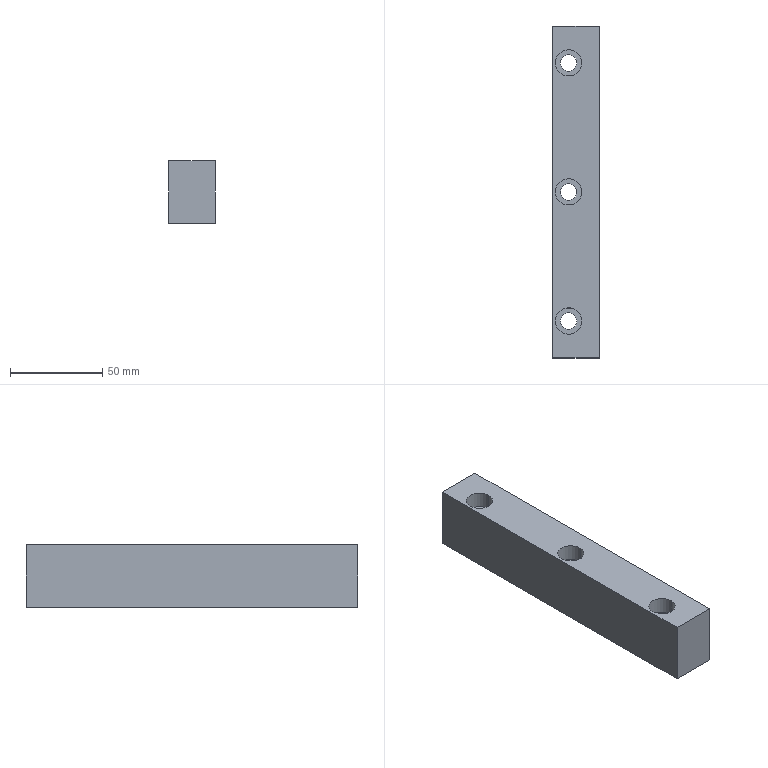Part | Creo | 1 solid | 21 faces | box 25 x 180 x 34 mm | volume 143923 mm3 | cylinder 12 | plane 9 | commonest cylinder face diameters 9 x6 14.25 x6
STEP:
#1=CARTESIAN_POINT('',(0.,0.,0.));
#2=DIRECTION('',(0.,0.,1.));
#3=DIRECTION('',(1.,0.,0.));
#4=AXIS2_PLACEMENT_3D('',#1,#2,#3);
#5=CARTESIAN_POINT('',(148.764,125.373,-29.441));
#6=VERTEX_POINT('',#5);
#7=CARTESIAN_POINT('',(173.764,125.373,-29.441));
#8=VERTEX_POINT('',#7);
#9=CARTESIAN_POINT('',(148.764,125.373,-29.441));
#10=DIRECTION('',(1.,0.,0.));
#11=VECTOR('',#10,25.);
#12=LINE('',#9,#11);
#13=EDGE_CURVE('',#6,#8,#12,.T.);
#14=ORIENTED_EDGE('',*,*,#13,.F.);
#15=CARTESIAN_POINT('',(148.764,305.373,-29.441));
#16=VERTEX_POINT('',#15);
#17=CARTESIAN_POINT('',(148.764,125.373,-29.441));
#18=DIRECTION('',(0.,1.,0.));
#19=VECTOR('',#18,180.);
#20=LINE('',#17,#19);
#21=EDGE_CURVE('',#6,#16,#20,.T.);
#22=ORIENTED_EDGE('',*,*,#21,.T.);
#23=CARTESIAN_POINT('',(173.764,305.373,-29.441));
#24=VERTEX_POINT('',#23);
#25=CARTESIAN_POINT('',(148.764,305.373,-29.441));
#26=DIRECTION('',(1.,0.,0.));
#27=VECTOR('',#26,25.);
#28=LINE('',#25,#27);
#29=EDGE_CURVE('',#16,#24,#28,.T.);
#30=ORIENTED_EDGE('',*,*,#29,.T.);
#31=CARTESIAN_POINT('',(173.764,125.373,-29.441));
#32=DIRECTION('',(0.,1.,0.));
#33=VECTOR('',#32,180.);
#34=LINE('',#31,#33);
#35=EDGE_CURVE('',#8,#24,#34,.T.);
#36=ORIENTED_EDGE('',*,*,#35,.F.);
#37=EDGE_LOOP('',(#14,#22,#30,#36));
#38=FACE_OUTER_BOUND('',#37,.F.);
#39=CARTESIAN_POINT('',(150.139,285.373,-29.441));
#40=VERTEX_POINT('',#39);
#41=CARTESIAN_POINT('',(164.389,285.373,-29.441));
#42=VERTEX_POINT('',#41);
#43=CARTESIAN_POINT('',(157.264,285.373,-29.441));
#44=DIRECTION('',(0.,0.,-1.));
#45=DIRECTION('',(-1.,0.,0.));
#46=AXIS2_PLACEMENT_3D('',#43,#44,#45);
#47=CIRCLE('',#46,7.125);
#48=EDGE_CURVE('',#40,#42,#47,.T.);
#49=ORIENTED_EDGE('',*,*,#48,.F.);
#50=CARTESIAN_POINT('',(157.264,285.373,-29.441));
#51=DIRECTION('',(0.,0.,-1.));
#52=DIRECTION('',(1.,0.,0.));
#53=AXIS2_PLACEMENT_3D('',#50,#51,#52);
#54=CIRCLE('',#53,7.125);
#55=EDGE_CURVE('',#42,#40,#54,.T.);
#56=ORIENTED_EDGE('',*,*,#55,.F.);
#57=EDGE_LOOP('',(#49,#56));
#58=FACE_BOUND('',#57,.F.);
#59=CARTESIAN_POINT('',(150.139,145.373,-29.441));
#60=VERTEX_POINT('',#59);
#61=CARTESIAN_POINT('',(164.389,145.373,-29.441));
#62=VERTEX_POINT('',#61);
#63=CARTESIAN_POINT('',(157.264,145.373,-29.441));
#64=DIRECTION('',(0.,0.,-1.));
#65=DIRECTION('',(-1.,0.,0.));
#66=AXIS2_PLACEMENT_3D('',#63,#64,#65);
#67=CIRCLE('',#66,7.125);
#68=EDGE_CURVE('',#60,#62,#67,.T.);
#69=ORIENTED_EDGE('',*,*,#68,.F.);
#70=CARTESIAN_POINT('',(157.264,145.373,-29.441));
#71=DIRECTION('',(0.,0.,-1.));
#72=DIRECTION('',(1.,0.,0.));
#73=AXIS2_PLACEMENT_3D('',#70,#71,#72);
#74=CIRCLE('',#73,7.125);
#75=EDGE_CURVE('',#62,#60,#74,.T.);
#76=ORIENTED_EDGE('',*,*,#75,.F.);
#77=EDGE_LOOP('',(#69,#76));
#78=FACE_BOUND('',#77,.F.);
#79=CARTESIAN_POINT('',(150.139,215.373,-29.441));
#80=VERTEX_POINT('',#79);
#81=CARTESIAN_POINT('',(164.389,215.373,-29.441));
#82=VERTEX_POINT('',#81);
#83=CARTESIAN_POINT('',(157.264,215.373,-29.441));
#84=DIRECTION('',(0.,0.,-1.));
#85=DIRECTION('',(-1.,0.,0.));
#86=AXIS2_PLACEMENT_3D('',#83,#84,#85);
#87=CIRCLE('',#86,7.125);
#88=EDGE_CURVE('',#80,#82,#87,.T.);
#89=ORIENTED_EDGE('',*,*,#88,.F.);
#90=CARTESIAN_POINT('',(157.264,215.373,-29.441));
#91=DIRECTION('',(0.,0.,-1.));
#92=DIRECTION('',(1.,0.,0.));
#93=AXIS2_PLACEMENT_3D('',#90,#91,#92);
#94=CIRCLE('',#93,7.125);
#95=EDGE_CURVE('',#82,#80,#94,.T.);
#96=ORIENTED_EDGE('',*,*,#95,.F.);
#97=EDGE_LOOP('',(#89,#96));
#98=FACE_BOUND('',#97,.F.);
#99=CARTESIAN_POINT('',(439.623,319.968,-29.441));
#100=DIRECTION('',(0.,0.,-1.));
#101=DIRECTION('',(-1.,0.,0.));
#102=AXIS2_PLACEMENT_3D('',#99,#100,#101);
#103=PLANE('',#102);
#104=ADVANCED_FACE('',(#38,#58,#78,#98),#103,.F.);
#105=ORIENTED_EDGE('',*,*,#48,.T.);
#106=CARTESIAN_POINT('',(164.389,285.373,-38.441));
#107=VERTEX_POINT('',#106);
#108=CARTESIAN_POINT('',(164.389,285.373,-38.441));
#109=DIRECTION('',(0.,0.,1.));
#110=VECTOR('',#109,9.);
#111=LINE('',#108,#110);
#112=EDGE_CURVE('',#107,#42,#111,.T.);
#113=ORIENTED_EDGE('',*,*,#112,.F.);
#114=CARTESIAN_POINT('',(150.139,285.373,-38.441));
#115=VERTEX_POINT('',#114);
#116=CARTESIAN_POINT('',(157.264,285.373,-38.441));
#117=DIRECTION('',(0.,0.,1.));
#118=DIRECTION('',(1.,0.,0.));
#119=AXIS2_PLACEMENT_3D('',#116,#117,#118);
#120=CIRCLE('',#119,7.125);
#121=EDGE_CURVE('',#107,#115,#120,.T.);
#122=ORIENTED_EDGE('',*,*,#121,.T.);
#123=CARTESIAN_POINT('',(150.139,285.373,-38.441));
#124=DIRECTION('',(0.,0.,1.));
#125=VECTOR('',#124,9.);
#126=LINE('',#123,#125);
#127=EDGE_CURVE('',#115,#40,#126,.T.);
#128=ORIENTED_EDGE('',*,*,#127,.T.);
#129=EDGE_LOOP('',(#105,#113,#122,#128));
#130=FACE_OUTER_BOUND('',#129,.F.);
#131=CARTESIAN_POINT('',(157.264,285.373,-38.441));
#132=DIRECTION('',(0.,0.,1.));
#133=DIRECTION('',(1.,0.,0.));
#134=AXIS2_PLACEMENT_3D('',#131,#132,#133);
#135=CYLINDRICAL_SURFACE('',#134,7.125);
#136=ADVANCED_FACE('',(#130),#135,.F.);
#137=ORIENTED_EDGE('',*,*,#55,.T.);
#138=ORIENTED_EDGE('',*,*,#127,.F.);
#139=CARTESIAN_POINT('',(157.264,285.373,-38.441));
#140=DIRECTION('',(0.,0.,1.));
#141=DIRECTION('',(-1.,0.,0.));
#142=AXIS2_PLACEMENT_3D('',#139,#140,#141);
#143=CIRCLE('',#142,7.125);
#144=EDGE_CURVE('',#115,#107,#143,.T.);
#145=ORIENTED_EDGE('',*,*,#144,.T.);
#146=ORIENTED_EDGE('',*,*,#112,.T.);
#147=EDGE_LOOP('',(#137,#138,#145,#146));
#148=FACE_OUTER_BOUND('',#147,.F.);
#149=CARTESIAN_POINT('',(157.264,285.373,-38.441));
#150=DIRECTION('',(0.,0.,1.));
#151=DIRECTION('',(1.,0.,0.));
#152=AXIS2_PLACEMENT_3D('',#149,#150,#151);
#153=CYLINDRICAL_SURFACE('',#152,7.125);
#154=ADVANCED_FACE('',(#148),#153,.F.);
#155=ORIENTED_EDGE('',*,*,#144,.F.);
#156=ORIENTED_EDGE('',*,*,#121,.F.);
#157=EDGE_LOOP('',(#155,#156));
#158=FACE_OUTER_BOUND('',#157,.F.);
#159=CARTESIAN_POINT('',(161.764,285.373,-38.441));
#160=VERTEX_POINT('',#159);
#161=CARTESIAN_POINT('',(152.764,285.373,-38.441));
#162=VERTEX_POINT('',#161);
#163=CARTESIAN_POINT('',(157.264,285.373,-38.441));
#164=DIRECTION('',(0.,0.,-1.));
#165=DIRECTION('',(1.,0.,0.));
#166=AXIS2_PLACEMENT_3D('',#163,#164,#165);
#167=CIRCLE('',#166,4.5);
#168=EDGE_CURVE('',#160,#162,#167,.T.);
#169=ORIENTED_EDGE('',*,*,#168,.F.);
#170=CARTESIAN_POINT('',(157.264,285.373,-38.441));
#171=DIRECTION('',(0.,0.,-1.));
#172=DIRECTION('',(-1.,0.,0.));
#173=AXIS2_PLACEMENT_3D('',#170,#171,#172);
#174=CIRCLE('',#173,4.5);
#175=EDGE_CURVE('',#162,#160,#174,.T.);
#176=ORIENTED_EDGE('',*,*,#175,.F.);
#177=EDGE_LOOP('',(#169,#176));
#178=FACE_BOUND('',#177,.F.);
#179=CARTESIAN_POINT('',(157.264,285.373,-38.441));
#180=DIRECTION('',(0.,0.,-1.));
#181=DIRECTION('',(-1.,0.,0.));
#182=AXIS2_PLACEMENT_3D('',#179,#180,#181);
#183=PLANE('',#182);
#184=ADVANCED_FACE('',(#158,#178),#183,.F.);
#185=CARTESIAN_POINT('',(152.764,285.373,-63.441));
#186=VERTEX_POINT('',#185);
#187=CARTESIAN_POINT('',(161.764,285.373,-63.441));
#188=VERTEX_POINT('',#187);
#189=CARTESIAN_POINT('',(157.264,285.373,-63.441));
#190=DIRECTION('',(0.,0.,1.));
#191=DIRECTION('',(-1.,0.,0.));
#192=AXIS2_PLACEMENT_3D('',#189,#190,#191);
#193=CIRCLE('',#192,4.5);
#194=EDGE_CURVE('',#186,#188,#193,.T.);
#195=ORIENTED_EDGE('',*,*,#194,.T.);
#196=CARTESIAN_POINT('',(161.764,285.373,-38.441));
#197=DIRECTION('',(0.,0.,-1.));
#198=VECTOR('',#197,25.);
#199=LINE('',#196,#198);
#200=EDGE_CURVE('',#160,#188,#199,.T.);
#201=ORIENTED_EDGE('',*,*,#200,.F.);
#202=ORIENTED_EDGE('',*,*,#168,.T.);
#203=CARTESIAN_POINT('',(152.764,285.373,-38.441));
#204=DIRECTION('',(0.,0.,-1.));
#205=VECTOR('',#204,25.);
#206=LINE('',#203,#205);
#207=EDGE_CURVE('',#162,#186,#206,.T.);
#208=ORIENTED_EDGE('',*,*,#207,.T.);
#209=EDGE_LOOP('',(#195,#201,#202,#208));
#210=FACE_OUTER_BOUND('',#209,.F.);
#211=CARTESIAN_POINT('',(157.264,285.373,-38.441));
#212=DIRECTION('',(0.,0.,-1.));
#213=DIRECTION('',(-1.,0.,0.));
#214=AXIS2_PLACEMENT_3D('',#211,#212,#213);
#215=CYLINDRICAL_SURFACE('',#214,4.5);
#216=ADVANCED_FACE('',(#210),#215,.F.);
#217=CARTESIAN_POINT('',(148.764,125.373,-63.441));
#218=VERTEX_POINT('',#217);
#219=CARTESIAN_POINT('',(173.764,125.373,-63.441));
#220=VERTEX_POINT('',#219);
#221=CARTESIAN_POINT('',(148.764,125.373,-63.441));
#222=DIRECTION('',(1.,0.,0.));
#223=VECTOR('',#222,25.);
#224=LINE('',#221,#223);
#225=EDGE_CURVE('',#218,#220,#224,.T.);
#226=ORIENTED_EDGE('',*,*,#225,.T.);
#227=CARTESIAN_POINT('',(173.764,305.373,-63.441));
#228=VERTEX_POINT('',#227);
#229=CARTESIAN_POINT('',(173.764,125.373,-63.441));
#230=DIRECTION('',(0.,1.,0.));
#231=VECTOR('',#230,180.);
#232=LINE('',#229,#231);
#233=EDGE_CURVE('',#220,#228,#232,.T.);
#234=ORIENTED_EDGE('',*,*,#233,.T.);
#235=CARTESIAN_POINT('',(148.764,305.373,-63.441));
#236=VERTEX_POINT('',#235);
#237=CARTESIAN_POINT('',(148.764,305.373,-63.441));
#238=DIRECTION('',(1.,0.,0.));
#239=VECTOR('',#238,25.);
#240=LINE('',#237,#239);
#241=EDGE_CURVE('',#236,#228,#240,.T.);
#242=ORIENTED_EDGE('',*,*,#241,.F.);
#243=CARTESIAN_POINT('',(148.764,125.373,-63.441));
#244=DIRECTION('',(0.,1.,0.));
#245=VECTOR('',#244,180.);
#246=LINE('',#243,#245);
#247=EDGE_CURVE('',#218,#236,#246,.T.);
#248=ORIENTED_EDGE('',*,*,#247,.F.);
#249=EDGE_LOOP('',(#226,#234,#242,#248));
#250=FACE_OUTER_BOUND('',#249,.F.);
#251=CARTESIAN_POINT('',(157.264,285.373,-63.441));
#252=DIRECTION('',(0.,0.,1.));
#253=DIRECTION('',(1.,0.,0.));
#254=AXIS2_PLACEMENT_3D('',#251,#252,#253);
#255=CIRCLE('',#254,4.5);
#256=EDGE_CURVE('',#188,#186,#255,.T.);
#257=ORIENTED_EDGE('',*,*,#256,.F.);
#258=ORIENTED_EDGE('',*,*,#194,.F.);
#259=EDGE_LOOP('',(#257,#258));
#260=FACE_BOUND('',#259,.F.);
#261=CARTESIAN_POINT('',(161.764,145.373,-63.441));
#262=VERTEX_POINT('',#261);
#263=CARTESIAN_POINT('',(152.764,145.373,-63.441));
#264=VERTEX_POINT('',#263);
#265=CARTESIAN_POINT('',(157.264,145.373,-63.441));
#266=DIRECTION('',(0.,0.,1.));
#267=DIRECTION('',(1.,0.,0.));
#268=AXIS2_PLACEMENT_3D('',#265,#266,#267);
#269=CIRCLE('',#268,4.5);
#270=EDGE_CURVE('',#262,#264,#269,.T.);
#271=ORIENTED_EDGE('',*,*,#270,.F.);
#272=CARTESIAN_POINT('',(157.264,145.373,-63.441));
#273=DIRECTION('',(0.,0.,1.));
#274=DIRECTION('',(-1.,0.,0.));
#275=AXIS2_PLACEMENT_3D('',#272,#273,#274);
#276=CIRCLE('',#275,4.5);
#277=EDGE_CURVE('',#264,#262,#276,.T.);
#278=ORIENTED_EDGE('',*,*,#277,.F.);
#279=EDGE_LOOP('',(#271,#278));
#280=FACE_BOUND('',#279,.F.);
#281=CARTESIAN_POINT('',(161.764,215.373,-63.441));
#282=VERTEX_POINT('',#281);
#283=CARTESIAN_POINT('',(152.764,215.373,-63.441));
#284=VERTEX_POINT('',#283);
#285=CARTESIAN_POINT('',(157.264,215.373,-63.441));
#286=DIRECTION('',(0.,0.,1.));
#287=DIRECTION('',(1.,0.,0.));
#288=AXIS2_PLACEMENT_3D('',#285,#286,#287);
#289=CIRCLE('',#288,4.5);
#290=EDGE_CURVE('',#282,#284,#289,.T.);
#291=ORIENTED_EDGE('',*,*,#290,.F.);
#292=CARTESIAN_POINT('',(157.264,215.373,-63.441));
#293=DIRECTION('',(0.,0.,1.));
#294=DIRECTION('',(-1.,0.,0.));
#295=AXIS2_PLACEMENT_3D('',#292,#293,#294);
#296=CIRCLE('',#295,4.5);
#297=EDGE_CURVE('',#284,#282,#296,.T.);
#298=ORIENTED_EDGE('',*,*,#297,.F.);
#299=EDGE_LOOP('',(#291,#298));
#300=FACE_BOUND('',#299,.F.);
#301=CARTESIAN_POINT('',(439.623,319.968,-63.441));
#302=DIRECTION('',(0.,0.,-1.));
#303=DIRECTION('',(-1.,0.,0.));
#304=AXIS2_PLACEMENT_3D('',#301,#302,#303);
#305=PLANE('',#304);
#306=ADVANCED_FACE('',(#250,#260,#280,#300),#305,.T.);
#307=ORIENTED_EDGE('',*,*,#290,.T.);
#308=CARTESIAN_POINT('',(152.764,215.373,-38.441));
#309=VERTEX_POINT('',#308);
#310=CARTESIAN_POINT('',(152.764,215.373,-38.441));
#311=DIRECTION('',(0.,0.,-1.));
#312=VECTOR('',#311,25.);
#313=LINE('',#310,#312);
#314=EDGE_CURVE('',#309,#284,#313,.T.);
#315=ORIENTED_EDGE('',*,*,#314,.F.);
#316=CARTESIAN_POINT('',(161.764,215.373,-38.441));
#317=VERTEX_POINT('',#316);
#318=CARTESIAN_POINT('',(157.264,215.373,-38.441));
#319=DIRECTION('',(0.,0.,-1.));
#320=DIRECTION('',(-1.,0.,0.));
#321=AXIS2_PLACEMENT_3D('',#318,#319,#320);
#322=CIRCLE('',#321,4.5);
#323=EDGE_CURVE('',#309,#317,#322,.T.);
#324=ORIENTED_EDGE('',*,*,#323,.T.);
#325=CARTESIAN_POINT('',(161.764,215.373,-38.441));
#326=DIRECTION('',(0.,0.,-1.));
#327=VECTOR('',#326,25.);
#328=LINE('',#325,#327);
#329=EDGE_CURVE('',#317,#282,#328,.T.);
#330=ORIENTED_EDGE('',*,*,#329,.T.);
#331=EDGE_LOOP('',(#307,#315,#324,#330));
#332=FACE_OUTER_BOUND('',#331,.F.);
#333=CARTESIAN_POINT('',(157.264,215.373,-38.441));
#334=DIRECTION('',(0.,0.,-1.));
#335=DIRECTION('',(-1.,0.,0.));
#336=AXIS2_PLACEMENT_3D('',#333,#334,#335);
#337=CYLINDRICAL_SURFACE('',#336,4.5);
#338=ADVANCED_FACE('',(#332),#337,.F.);
#339=ORIENTED_EDGE('',*,*,#297,.T.);
#340=ORIENTED_EDGE('',*,*,#329,.F.);
#341=CARTESIAN_POINT('',(157.264,215.373,-38.441));
#342=DIRECTION('',(0.,0.,-1.));
#343=DIRECTION('',(1.,0.,0.));
#344=AXIS2_PLACEMENT_3D('',#341,#342,#343);
#345=CIRCLE('',#344,4.5);
#346=EDGE_CURVE('',#317,#309,#345,.T.);
#347=ORIENTED_EDGE('',*,*,#346,.T.);
#348=ORIENTED_EDGE('',*,*,#314,.T.);
#349=EDGE_LOOP('',(#339,#340,#347,#348));
#350=FACE_OUTER_BOUND('',#349,.F.);
#351=CARTESIAN_POINT('',(157.264,215.373,-38.441));
#352=DIRECTION('',(0.,0.,-1.));
#353=DIRECTION('',(-1.,0.,0.));
#354=AXIS2_PLACEMENT_3D('',#351,#352,#353);
#355=CYLINDRICAL_SURFACE('',#354,4.5);
#356=ADVANCED_FACE('',(#350),#355,.F.);
#357=CARTESIAN_POINT('',(150.139,215.373,-38.441));
#358=VERTEX_POINT('',#357);
#359=CARTESIAN_POINT('',(164.389,215.373,-38.441));
#360=VERTEX_POINT('',#359);
#361=CARTESIAN_POINT('',(157.264,215.373,-38.441));
#362=DIRECTION('',(0.,0.,1.));
#363=DIRECTION('',(-1.,0.,0.));
#364=AXIS2_PLACEMENT_3D('',#361,#362,#363);
#365=CIRCLE('',#364,7.125);
#366=EDGE_CURVE('',#358,#360,#365,.T.);
#367=ORIENTED_EDGE('',*,*,#366,.F.);
#368=CARTESIAN_POINT('',(157.264,215.373,-38.441));
#369=DIRECTION('',(0.,0.,1.));
#370=DIRECTION('',(1.,0.,0.));
#371=AXIS2_PLACEMENT_3D('',#368,#369,#370);
#372=CIRCLE('',#371,7.125);
#373=EDGE_CURVE('',#360,#358,#372,.T.);
#374=ORIENTED_EDGE('',*,*,#373,.F.);
#375=EDGE_LOOP('',(#367,#374));
#376=FACE_OUTER_BOUND('',#375,.F.);
#377=ORIENTED_EDGE('',*,*,#346,.F.);
#378=ORIENTED_EDGE('',*,*,#323,.F.);
#379=EDGE_LOOP('',(#377,#378));
#380=FACE_BOUND('',#379,.F.);
#381=CARTESIAN_POINT('',(157.264,215.373,-38.441));
#382=DIRECTION('',(0.,0.,-1.));
#383=DIRECTION('',(-1.,0.,0.));
#384=AXIS2_PLACEMENT_3D('',#381,#382,#383);
#385=PLANE('',#384);
#386=ADVANCED_FACE('',(#376,#380),#385,.F.);
#387=ORIENTED_EDGE('',*,*,#95,.T.);
#388=CARTESIAN_POINT('',(150.139,215.373,-38.441));
#389=DIRECTION('',(0.,0.,1.));
#390=VECTOR('',#389,9.);
#391=LINE('',#388,#390);
#392=EDGE_CURVE('',#358,#80,#391,.T.);
#393=ORIENTED_EDGE('',*,*,#392,.F.);
#394=ORIENTED_EDGE('',*,*,#366,.T.);
#395=CARTESIAN_POINT('',(164.389,215.373,-38.441));
#396=DIRECTION('',(0.,0.,1.));
#397=VECTOR('',#396,9.);
#398=LINE('',#395,#397);
#399=EDGE_CURVE('',#360,#82,#398,.T.);
#400=ORIENTED_EDGE('',*,*,#399,.T.);
#401=EDGE_LOOP('',(#387,#393,#394,#400));
#402=FACE_OUTER_BOUND('',#401,.F.);
#403=CARTESIAN_POINT('',(157.264,215.373,-38.441));
#404=DIRECTION('',(0.,0.,1.));
#405=DIRECTION('',(1.,0.,0.));
#406=AXIS2_PLACEMENT_3D('',#403,#404,#405);
#407=CYLINDRICAL_SURFACE('',#406,7.125);
#408=ADVANCED_FACE('',(#402),#407,.F.);
#409=ORIENTED_EDGE('',*,*,#88,.T.);
#410=ORIENTED_EDGE('',*,*,#399,.F.);
#411=ORIENTED_EDGE('',*,*,#373,.T.);
#412=ORIENTED_EDGE('',*,*,#392,.T.);
#413=EDGE_LOOP('',(#409,#410,#411,#412));
#414=FACE_OUTER_BOUND('',#413,.F.);
#415=CARTESIAN_POINT('',(157.264,215.373,-38.441));
#416=DIRECTION('',(0.,0.,1.));
#417=DIRECTION('',(1.,0.,0.));
#418=AXIS2_PLACEMENT_3D('',#415,#416,#417);
#419=CYLINDRICAL_SURFACE('',#418,7.125);
#420=ADVANCED_FACE('',(#414),#419,.F.);
#421=ORIENTED_EDGE('',*,*,#256,.T.);
#422=ORIENTED_EDGE('',*,*,#207,.F.);
#423=ORIENTED_EDGE('',*,*,#175,.T.);
#424=ORIENTED_EDGE('',*,*,#200,.T.);
#425=EDGE_LOOP('',(#421,#422,#423,#424));
#426=FACE_OUTER_BOUND('',#425,.F.);
#427=CARTESIAN_POINT('',(157.264,285.373,-38.441));
#428=DIRECTION('',(0.,0.,-1.));
#429=DIRECTION('',(-1.,0.,0.));
#430=AXIS2_PLACEMENT_3D('',#427,#428,#429);
#431=CYLINDRICAL_SURFACE('',#430,4.5);
#432=ADVANCED_FACE('',(#426),#431,.F.);
#433=ORIENTED_EDGE('',*,*,#270,.T.);
#434=CARTESIAN_POINT('',(152.764,145.373,-38.441));
#435=VERTEX_POINT('',#434);
#436=CARTESIAN_POINT('',(152.764,145.373,-38.441));
#437=DIRECTION('',(0.,0.,-1.));
#438=VECTOR('',#437,25.);
#439=LINE('',#436,#438);
#440=EDGE_CURVE('',#435,#264,#439,.T.);
#441=ORIENTED_EDGE('',*,*,#440,.F.);
#442=CARTESIAN_POINT('',(161.764,145.373,-38.441));
#443=VERTEX_POINT('',#442);
#444=CARTESIAN_POINT('',(157.264,145.373,-38.441));
#445=DIRECTION('',(0.,0.,-1.));
#446=DIRECTION('',(-1.,0.,0.));
#447=AXIS2_PLACEMENT_3D('',#444,#445,#446);
#448=CIRCLE('',#447,4.5);
#449=EDGE_CURVE('',#435,#443,#448,.T.);
#450=ORIENTED_EDGE('',*,*,#449,.T.);
#451=CARTESIAN_POINT('',(161.764,145.373,-38.441));
#452=DIRECTION('',(0.,0.,-1.));
#453=VECTOR('',#452,25.);
#454=LINE('',#451,#453);
#455=EDGE_CURVE('',#443,#262,#454,.T.);
#456=ORIENTED_EDGE('',*,*,#455,.T.);
#457=EDGE_LOOP('',(#433,#441,#450,#456));
#458=FACE_OUTER_BOUND('',#457,.F.);
#459=CARTESIAN_POINT('',(157.264,145.373,-38.441));
#460=DIRECTION('',(0.,0.,-1.));
#461=DIRECTION('',(-1.,0.,0.));
#462=AXIS2_PLACEMENT_3D('',#459,#460,#461);
#463=CYLINDRICAL_SURFACE('',#462,4.5);
#464=ADVANCED_FACE('',(#458),#463,.F.);
#465=ORIENTED_EDGE('',*,*,#277,.T.);
#466=ORIENTED_EDGE('',*,*,#455,.F.);
#467=CARTESIAN_POINT('',(157.264,145.373,-38.441));
#468=DIRECTION('',(0.,0.,-1.));
#469=DIRECTION('',(1.,0.,0.));
#470=AXIS2_PLACEMENT_3D('',#467,#468,#469);
#471=CIRCLE('',#470,4.5);
#472=EDGE_CURVE('',#443,#435,#471,.T.);
#473=ORIENTED_EDGE('',*,*,#472,.T.);
#474=ORIENTED_EDGE('',*,*,#440,.T.);
#475=EDGE_LOOP('',(#465,#466,#473,#474));
#476=FACE_OUTER_BOUND('',#475,.F.);
#477=CARTESIAN_POINT('',(157.264,145.373,-38.441));
#478=DIRECTION('',(0.,0.,-1.));
#479=DIRECTION('',(-1.,0.,0.));
#480=AXIS2_PLACEMENT_3D('',#477,#478,#479);
#481=CYLINDRICAL_SURFACE('',#480,4.5);
#482=ADVANCED_FACE('',(#476),#481,.F.);
#483=CARTESIAN_POINT('',(150.139,145.373,-38.441));
#484=VERTEX_POINT('',#483);
#485=CARTESIAN_POINT('',(164.389,145.373,-38.441));
#486=VERTEX_POINT('',#485);
#487=CARTESIAN_POINT('',(157.264,145.373,-38.441));
#488=DIRECTION('',(0.,0.,1.));
#489=DIRECTION('',(-1.,0.,0.));
#490=AXIS2_PLACEMENT_3D('',#487,#488,#489);
#491=CIRCLE('',#490,7.125);
#492=EDGE_CURVE('',#484,#486,#491,.T.);
#493=ORIENTED_EDGE('',*,*,#492,.F.);
#494=CARTESIAN_POINT('',(157.264,145.373,-38.441));
#495=DIRECTION('',(0.,0.,1.));
#496=DIRECTION('',(1.,0.,0.));
#497=AXIS2_PLACEMENT_3D('',#494,#495,#496);
#498=CIRCLE('',#497,7.125);
#499=EDGE_CURVE('',#486,#484,#498,.T.);
#500=ORIENTED_EDGE('',*,*,#499,.F.);
#501=EDGE_LOOP('',(#493,#500));
#502=FACE_OUTER_BOUND('',#501,.F.);
#503=ORIENTED_EDGE('',*,*,#472,.F.);
#504=ORIENTED_EDGE('',*,*,#449,.F.);
#505=EDGE_LOOP('',(#503,#504));
#506=FACE_BOUND('',#505,.F.);
#507=CARTESIAN_POINT('',(157.264,145.373,-38.441));
#508=DIRECTION('',(0.,0.,-1.));
#509=DIRECTION('',(-1.,0.,0.));
#510=AXIS2_PLACEMENT_3D('',#507,#508,#509);
#511=PLANE('',#510);
#512=ADVANCED_FACE('',(#502,#506),#511,.F.);
#513=ORIENTED_EDGE('',*,*,#75,.T.);
#514=CARTESIAN_POINT('',(150.139,145.373,-38.441));
#515=DIRECTION('',(0.,0.,1.));
#516=VECTOR('',#515,9.);
#517=LINE('',#514,#516);
#518=EDGE_CURVE('',#484,#60,#517,.T.);
#519=ORIENTED_EDGE('',*,*,#518,.F.);
#520=ORIENTED_EDGE('',*,*,#492,.T.);
#521=CARTESIAN_POINT('',(164.389,145.373,-38.441));
#522=DIRECTION('',(0.,0.,1.));
#523=VECTOR('',#522,9.);
#524=LINE('',#521,#523);
#525=EDGE_CURVE('',#486,#62,#524,.T.);
#526=ORIENTED_EDGE('',*,*,#525,.T.);
#527=EDGE_LOOP('',(#513,#519,#520,#526));
#528=FACE_OUTER_BOUND('',#527,.F.);
#529=CARTESIAN_POINT('',(157.264,145.373,-38.441));
#530=DIRECTION('',(0.,0.,1.));
#531=DIRECTION('',(1.,0.,0.));
#532=AXIS2_PLACEMENT_3D('',#529,#530,#531);
#533=CYLINDRICAL_SURFACE('',#532,7.125);
#534=ADVANCED_FACE('',(#528),#533,.F.);
#535=ORIENTED_EDGE('',*,*,#68,.T.);
#536=ORIENTED_EDGE('',*,*,#525,.F.);
#537=ORIENTED_EDGE('',*,*,#499,.T.);
#538=ORIENTED_EDGE('',*,*,#518,.T.);
#539=EDGE_LOOP('',(#535,#536,#537,#538));
#540=FACE_OUTER_BOUND('',#539,.F.);
#541=CARTESIAN_POINT('',(157.264,145.373,-38.441));
#542=DIRECTION('',(0.,0.,1.));
#543=DIRECTION('',(1.,0.,0.));
#544=AXIS2_PLACEMENT_3D('',#541,#542,#543);
#545=CYLINDRICAL_SURFACE('',#544,7.125);
#546=ADVANCED_FACE('',(#540),#545,.F.);
#547=CARTESIAN_POINT('',(173.764,125.373,-29.441));
#548=DIRECTION('',(0.,0.,-1.));
#549=VECTOR('',#548,34.);
#550=LINE('',#547,#549);
#551=EDGE_CURVE('',#8,#220,#550,.T.);
#552=ORIENTED_EDGE('',*,*,#551,.T.);
#553=ORIENTED_EDGE('',*,*,#225,.F.);
#554=CARTESIAN_POINT('',(148.764,125.373,-29.441));
#555=DIRECTION('',(0.,0.,-1.));
#556=VECTOR('',#555,34.);
#557=LINE('',#554,#556);
#558=EDGE_CURVE('',#6,#218,#557,.T.);
#559=ORIENTED_EDGE('',*,*,#558,.F.);
#560=ORIENTED_EDGE('',*,*,#13,.T.);
#561=EDGE_LOOP('',(#552,#553,#559,#560));
#562=FACE_OUTER_BOUND('',#561,.F.);
#563=CARTESIAN_POINT('',(222.674,125.373,-63.441));
#564=DIRECTION('',(0.,1.,0.));
#565=DIRECTION('',(0.,0.,1.));
#566=AXIS2_PLACEMENT_3D('',#563,#564,#565);
#567=PLANE('',#566);
#568=ADVANCED_FACE('',(#562),#567,.F.);
#569=CARTESIAN_POINT('',(173.764,305.373,-29.441));
#570=DIRECTION('',(0.,0.,-1.));
#571=VECTOR('',#570,34.);
#572=LINE('',#569,#571);
#573=EDGE_CURVE('',#24,#228,#572,.T.);
#574=ORIENTED_EDGE('',*,*,#573,.T.);
#575=ORIENTED_EDGE('',*,*,#233,.F.);
#576=ORIENTED_EDGE('',*,*,#551,.F.);
#577=ORIENTED_EDGE('',*,*,#35,.T.);
#578=EDGE_LOOP('',(#574,#575,#576,#577));
#579=FACE_OUTER_BOUND('',#578,.F.);
#580=CARTESIAN_POINT('',(173.764,319.968,-63.441));
#581=DIRECTION('',(-1.,0.,0.));
#582=DIRECTION('',(0.,0.,1.));
#583=AXIS2_PLACEMENT_3D('',#580,#581,#582);
#584=PLANE('',#583);
#585=ADVANCED_FACE('',(#579),#584,.F.);
#586=CARTESIAN_POINT('',(148.764,305.373,-29.441));
#587=DIRECTION('',(0.,0.,-1.));
#588=VECTOR('',#587,34.);
#589=LINE('',#586,#588);
#590=EDGE_CURVE('',#16,#236,#589,.T.);
#591=ORIENTED_EDGE('',*,*,#590,.T.);
#592=ORIENTED_EDGE('',*,*,#241,.T.);
#593=ORIENTED_EDGE('',*,*,#573,.F.);
#594=ORIENTED_EDGE('',*,*,#29,.F.);
#595=EDGE_LOOP('',(#591,#592,#593,#594));
#596=FACE_OUTER_BOUND('',#595,.F.);
#597=CARTESIAN_POINT('',(439.623,305.373,-63.441));
#598=DIRECTION('',(0.,-1.,0.));
#599=DIRECTION('',(1.,0.,0.));
#600=AXIS2_PLACEMENT_3D('',#597,#598,#599);
#601=PLANE('',#600);
#602=ADVANCED_FACE('',(#596),#601,.F.);
#603=ORIENTED_EDGE('',*,*,#247,.T.);
#604=ORIENTED_EDGE('',*,*,#590,.F.);
#605=ORIENTED_EDGE('',*,*,#21,.F.);
#606=ORIENTED_EDGE('',*,*,#558,.T.);
#607=EDGE_LOOP('',(#603,#604,#605,#606));
#608=FACE_OUTER_BOUND('',#607,.F.);
#609=CARTESIAN_POINT('',(148.764,250.373,-63.441));
#610=DIRECTION('',(-1.,0.,0.));
#611=DIRECTION('',(0.,0.,1.));
#612=AXIS2_PLACEMENT_3D('',#609,#610,#611);
#613=PLANE('',#612);
#614=ADVANCED_FACE('',(#608),#613,.T.);
#615=CLOSED_SHELL('',(#104,#136,#154,#184,#216,#306,#338,#356,#386,#408,#420,#432,#464,#482,#512,#534,#546,#568,#585,#602,#614));
#616=MANIFOLD_SOLID_BREP('',#615);
#617=(LENGTH_UNIT()NAMED_UNIT(*)SI_UNIT(.MILLI.,.METRE.));
#618=UNCERTAINTY_MEASURE_WITH_UNIT(LENGTH_MEASURE(0.01849),#617,'','');
#619=(NAMED_UNIT(*)PLANE_ANGLE_UNIT()SI_UNIT($,.RADIAN.));
#620=PLANE_ANGLE_MEASURE_WITH_UNIT(PLANE_ANGLE_MEASURE(0.01745),#619);
#621=(CONVERSION_BASED_UNIT('DEGREE',#620)NAMED_UNIT(*)PLANE_ANGLE_UNIT());
#622=(NAMED_UNIT(*)SI_UNIT($,.STERADIAN.)SOLID_ANGLE_UNIT());
#623=(GEOMETRIC_REPRESENTATION_CONTEXT(3)GLOBAL_UNCERTAINTY_ASSIGNED_CONTEXT((#618))GLOBAL_UNIT_ASSIGNED_CONTEXT((#617,#621,#622))REPRESENTATION_CONTEXT('',''));
#624=ADVANCED_BREP_SHAPE_REPRESENTATION('',(#4,#616),#623);